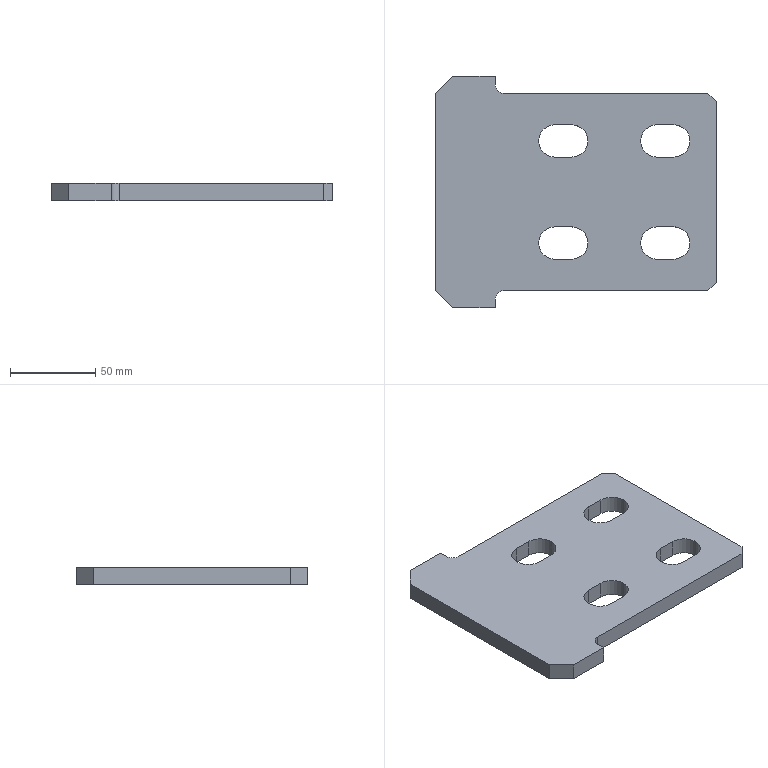Part | STEP file | 筋Plate-150×75-150 | 1 solid | 36 faces | box 165 x 136 x 10 mm | volume 178316 mm3 | plane 22 | cylinder 14 | commonest cylinder face diameters 19 x12 10 x2